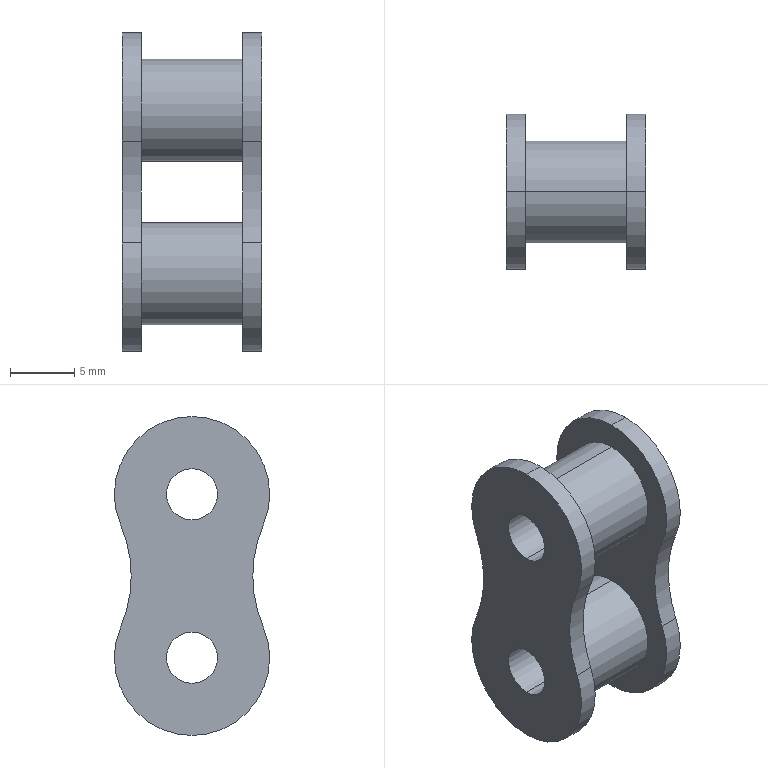Part | SolidWorks | features MoveFace 4, BaseBody 1, DelFace 1 | 1 solid | 22 faces | box 10.85 x 12.07 x 24.77 mm | volume 1258 mm3 | cylinder 18 | plane 4 | commonest cylinder face diameters 12.07 x6 3.98 x4 7.95 x4 20 x4
STEP:
#1=CARTESIAN_POINT('',(3.925,0.,3.975));
#2=VERTEX_POINT('',#1);
#3=CARTESIAN_POINT('',(3.925,0.,-3.975));
#4=VERTEX_POINT('',#3);
#5=CARTESIAN_POINT('',(3.925,0.,0.));
#6=DIRECTION('',(1.,0.,0.));
#7=DIRECTION('',(0.,0.,-1.));
#8=AXIS2_PLACEMENT_3D('',#5,#6,#7);
#9=CIRCLE('',#8,3.975);
#10=EDGE_CURVE('',#2,#4,#9,.T.);
#11=ORIENTED_EDGE('',*,*,#10,.F.);
#12=CARTESIAN_POINT('',(-3.925,0.,3.975));
#13=VERTEX_POINT('',#12);
#14=CARTESIAN_POINT('',(50.,0.,3.975));
#15=DIRECTION('',(-1.,0.,0.));
#16=VECTOR('',#15,1000.);
#17=LINE('',#14,#16);
#18=EDGE_CURVE('',#2,#13,#17,.T.);
#19=ORIENTED_EDGE('',*,*,#18,.T.);
#20=CARTESIAN_POINT('',(-3.925,0.,-3.975));
#21=VERTEX_POINT('',#20);
#22=CARTESIAN_POINT('',(-3.925,0.,0.));
#23=DIRECTION('',(1.,0.,0.));
#24=DIRECTION('',(0.,0.,-1.));
#25=AXIS2_PLACEMENT_3D('',#22,#23,#24);
#26=CIRCLE('',#25,3.975);
#27=EDGE_CURVE('',#13,#21,#26,.T.);
#28=ORIENTED_EDGE('',*,*,#27,.T.);
#29=CARTESIAN_POINT('',(50.,0.,-3.975));
#30=DIRECTION('',(-1.,0.,0.));
#31=VECTOR('',#30,1000.);
#32=LINE('',#29,#31);
#33=EDGE_CURVE('',#4,#21,#32,.T.);
#34=ORIENTED_EDGE('',*,*,#33,.F.);
#35=EDGE_LOOP('',(#11,#19,#28,#34));
#36=FACE_OUTER_BOUND('',#35,.T.);
#37=CARTESIAN_POINT('',(50.,0.,0.));
#38=DIRECTION('',(-1.,0.,0.));
#39=DIRECTION('',(0.,0.,-1.));
#40=AXIS2_PLACEMENT_3D('',#37,#38,#39);
#41=CYLINDRICAL_SURFACE('',#40,3.975);
#42=ADVANCED_FACE('',(#36),#41,.T.);
#43=CARTESIAN_POINT('',(3.925,0.,-8.725));
#44=VERTEX_POINT('',#43);
#45=CARTESIAN_POINT('',(3.925,0.,-16.675));
#46=VERTEX_POINT('',#45);
#47=CARTESIAN_POINT('',(3.925,0.,-12.7));
#48=DIRECTION('',(1.,0.,0.));
#49=DIRECTION('',(0.,0.,-1.));
#50=AXIS2_PLACEMENT_3D('',#47,#48,#49);
#51=CIRCLE('',#50,3.975);
#52=EDGE_CURVE('',#44,#46,#51,.T.);
#53=ORIENTED_EDGE('',*,*,#52,.F.);
#54=CARTESIAN_POINT('',(-3.925,0.,-8.725));
#55=VERTEX_POINT('',#54);
#56=CARTESIAN_POINT('',(50.,0.,-8.725));
#57=DIRECTION('',(-1.,0.,0.));
#58=VECTOR('',#57,1000.);
#59=LINE('',#56,#58);
#60=EDGE_CURVE('',#44,#55,#59,.T.);
#61=ORIENTED_EDGE('',*,*,#60,.T.);
#62=CARTESIAN_POINT('',(-3.925,0.,-16.675));
#63=VERTEX_POINT('',#62);
#64=CARTESIAN_POINT('',(-3.925,0.,-12.7));
#65=DIRECTION('',(1.,0.,0.));
#66=DIRECTION('',(0.,0.,-1.));
#67=AXIS2_PLACEMENT_3D('',#64,#65,#66);
#68=CIRCLE('',#67,3.975);
#69=EDGE_CURVE('',#55,#63,#68,.T.);
#70=ORIENTED_EDGE('',*,*,#69,.T.);
#71=CARTESIAN_POINT('',(50.,0.,-16.675));
#72=DIRECTION('',(-1.,0.,0.));
#73=VECTOR('',#72,1000.);
#74=LINE('',#71,#73);
#75=EDGE_CURVE('',#46,#63,#74,.T.);
#76=ORIENTED_EDGE('',*,*,#75,.F.);
#77=EDGE_LOOP('',(#53,#61,#70,#76));
#78=FACE_OUTER_BOUND('',#77,.T.);
#79=CARTESIAN_POINT('',(50.,0.,-12.7));
#80=DIRECTION('',(-1.,0.,0.));
#81=DIRECTION('',(0.,0.,-1.));
#82=AXIS2_PLACEMENT_3D('',#79,#80,#81);
#83=CYLINDRICAL_SURFACE('',#82,3.975);
#84=ADVANCED_FACE('',(#78),#83,.T.);
#85=CARTESIAN_POINT('',(-5.425,0.,-14.69));
#86=VERTEX_POINT('',#85);
#87=CARTESIAN_POINT('',(-5.425,0.,-10.71));
#88=VERTEX_POINT('',#87);
#89=CARTESIAN_POINT('',(-5.425,0.,-12.7));
#90=DIRECTION('',(1.,0.,0.));
#91=DIRECTION('',(0.,0.,-1.));
#92=AXIS2_PLACEMENT_3D('',#89,#90,#91);
#93=CIRCLE('',#92,1.99);
#94=EDGE_CURVE('',#86,#88,#93,.T.);
#95=ORIENTED_EDGE('',*,*,#94,.F.);
#96=CARTESIAN_POINT('',(5.425,0.,-14.69));
#97=VERTEX_POINT('',#96);
#98=CARTESIAN_POINT('',(5.925,0.,-14.69));
#99=DIRECTION('',(1.,0.,0.));
#100=VECTOR('',#99,1000.);
#101=LINE('',#98,#100);
#102=EDGE_CURVE('',#86,#97,#101,.T.);
#103=ORIENTED_EDGE('',*,*,#102,.T.);
#104=CARTESIAN_POINT('',(5.425,0.,-10.71));
#105=VERTEX_POINT('',#104);
#106=CARTESIAN_POINT('',(5.425,0.,-12.7));
#107=DIRECTION('',(1.,0.,0.));
#108=DIRECTION('',(0.,0.,-1.));
#109=AXIS2_PLACEMENT_3D('',#106,#107,#108);
#110=CIRCLE('',#109,1.99);
#111=EDGE_CURVE('',#97,#105,#110,.T.);
#112=ORIENTED_EDGE('',*,*,#111,.T.);
#113=CARTESIAN_POINT('',(5.925,0.,-10.71));
#114=DIRECTION('',(1.,0.,0.));
#115=VECTOR('',#114,1000.);
#116=LINE('',#113,#115);
#117=EDGE_CURVE('',#88,#105,#116,.T.);
#118=ORIENTED_EDGE('',*,*,#117,.F.);
#119=EDGE_LOOP('',(#95,#103,#112,#118));
#120=FACE_OUTER_BOUND('',#119,.T.);
#121=CARTESIAN_POINT('',(5.925,0.,-12.7));
#122=DIRECTION('',(1.,0.,0.));
#123=DIRECTION('',(0.,0.,1.));
#124=AXIS2_PLACEMENT_3D('',#121,#122,#123);
#125=CYLINDRICAL_SURFACE('',#124,1.99);
#126=ADVANCED_FACE('',(#120),#125,.F.);
#127=CARTESIAN_POINT('',(-5.425,0.,-1.99));
#128=VERTEX_POINT('',#127);
#129=CARTESIAN_POINT('',(-5.425,0.,1.99));
#130=VERTEX_POINT('',#129);
#131=CARTESIAN_POINT('',(-5.425,0.,0.));
#132=DIRECTION('',(1.,0.,0.));
#133=DIRECTION('',(0.,0.,-1.));
#134=AXIS2_PLACEMENT_3D('',#131,#132,#133);
#135=CIRCLE('',#134,1.99);
#136=EDGE_CURVE('',#128,#130,#135,.T.);
#137=ORIENTED_EDGE('',*,*,#136,.F.);
#138=CARTESIAN_POINT('',(5.425,0.,-1.99));
#139=VERTEX_POINT('',#138);
#140=CARTESIAN_POINT('',(5.925,0.,-1.99));
#141=DIRECTION('',(1.,0.,0.));
#142=VECTOR('',#141,1000.);
#143=LINE('',#140,#142);
#144=EDGE_CURVE('',#128,#139,#143,.T.);
#145=ORIENTED_EDGE('',*,*,#144,.T.);
#146=CARTESIAN_POINT('',(5.425,0.,1.99));
#147=VERTEX_POINT('',#146);
#148=CARTESIAN_POINT('',(5.425,0.,0.));
#149=DIRECTION('',(1.,0.,0.));
#150=DIRECTION('',(0.,0.,-1.));
#151=AXIS2_PLACEMENT_3D('',#148,#149,#150);
#152=CIRCLE('',#151,1.99);
#153=EDGE_CURVE('',#139,#147,#152,.T.);
#154=ORIENTED_EDGE('',*,*,#153,.T.);
#155=CARTESIAN_POINT('',(5.925,0.,1.99));
#156=DIRECTION('',(1.,0.,0.));
#157=VECTOR('',#156,1000.);
#158=LINE('',#155,#157);
#159=EDGE_CURVE('',#130,#147,#158,.T.);
#160=ORIENTED_EDGE('',*,*,#159,.F.);
#161=EDGE_LOOP('',(#137,#145,#154,#160));
#162=FACE_OUTER_BOUND('',#161,.T.);
#163=CARTESIAN_POINT('',(5.925,0.,0.));
#164=DIRECTION('',(1.,0.,0.));
#165=DIRECTION('',(0.,0.,1.));
#166=AXIS2_PLACEMENT_3D('',#163,#164,#165);
#167=CYLINDRICAL_SURFACE('',#166,1.99);
#168=ADVANCED_FACE('',(#162),#167,.F.);
#169=CARTESIAN_POINT('',(3.925,5.542,-2.39));
#170=VERTEX_POINT('',#169);
#171=CARTESIAN_POINT('',(3.925,0.,6.035));
#172=VERTEX_POINT('',#171);
#173=CARTESIAN_POINT('',(3.925,0.,0.));
#174=DIRECTION('',(1.,0.,0.));
#175=DIRECTION('',(0.,0.,-1.));
#176=AXIS2_PLACEMENT_3D('',#173,#174,#175);
#177=CIRCLE('',#176,6.035);
#178=EDGE_CURVE('',#170,#172,#177,.T.);
#179=ORIENTED_EDGE('',*,*,#178,.T.);
#180=CARTESIAN_POINT('',(5.425,0.,6.035));
#181=VERTEX_POINT('',#180);
#182=CARTESIAN_POINT('',(5.925,0.,6.035));
#183=DIRECTION('',(1.,0.,0.));
#184=VECTOR('',#183,1000.);
#185=LINE('',#182,#184);
#186=EDGE_CURVE('',#172,#181,#185,.T.);
#187=ORIENTED_EDGE('',*,*,#186,.T.);
#188=CARTESIAN_POINT('',(5.425,5.542,-2.39));
#189=VERTEX_POINT('',#188);
#190=CARTESIAN_POINT('',(5.425,0.,0.));
#191=DIRECTION('',(1.,0.,0.));
#192=DIRECTION('',(0.,0.,-1.));
#193=AXIS2_PLACEMENT_3D('',#190,#191,#192);
#194=CIRCLE('',#193,6.035);
#195=EDGE_CURVE('',#189,#181,#194,.T.);
#196=ORIENTED_EDGE('',*,*,#195,.F.);
#197=CARTESIAN_POINT('',(5.925,5.542,-2.39));
#198=DIRECTION('',(-1.,0.,0.));
#199=VECTOR('',#198,1000.);
#200=LINE('',#197,#199);
#201=EDGE_CURVE('',#189,#170,#200,.T.);
#202=ORIENTED_EDGE('',*,*,#201,.T.);
#203=EDGE_LOOP('',(#179,#187,#196,#202));
#204=FACE_OUTER_BOUND('',#203,.T.);
#205=CARTESIAN_POINT('',(5.925,0.,0.));
#206=DIRECTION('',(1.,0.,0.));
#207=DIRECTION('',(0.,0.,1.));
#208=AXIS2_PLACEMENT_3D('',#205,#206,#207);
#209=CYLINDRICAL_SURFACE('',#208,6.035);
#210=ADVANCED_FACE('',(#204),#209,.T.);
#211=CARTESIAN_POINT('',(-5.425,5.542,-2.39));
#212=VERTEX_POINT('',#211);
#213=CARTESIAN_POINT('',(-5.425,0.,6.035));
#214=VERTEX_POINT('',#213);
#215=CARTESIAN_POINT('',(-5.425,0.,0.));
#216=DIRECTION('',(1.,0.,0.));
#217=DIRECTION('',(0.,0.,-1.));
#218=AXIS2_PLACEMENT_3D('',#215,#216,#217);
#219=CIRCLE('',#218,6.035);
#220=EDGE_CURVE('',#212,#214,#219,.T.);
#221=ORIENTED_EDGE('',*,*,#220,.T.);
#222=CARTESIAN_POINT('',(-3.925,0.,6.035));
#223=VERTEX_POINT('',#222);
#224=CARTESIAN_POINT('',(5.925,0.,6.035));
#225=DIRECTION('',(1.,0.,0.));
#226=VECTOR('',#225,1000.);
#227=LINE('',#224,#226);
#228=EDGE_CURVE('',#214,#223,#227,.T.);
#229=ORIENTED_EDGE('',*,*,#228,.T.);
#230=CARTESIAN_POINT('',(-3.925,5.542,-2.39));
#231=VERTEX_POINT('',#230);
#232=CARTESIAN_POINT('',(-3.925,0.,0.));
#233=DIRECTION('',(1.,0.,0.));
#234=DIRECTION('',(0.,0.,-1.));
#235=AXIS2_PLACEMENT_3D('',#232,#233,#234);
#236=CIRCLE('',#235,6.035);
#237=EDGE_CURVE('',#231,#223,#236,.T.);
#238=ORIENTED_EDGE('',*,*,#237,.F.);
#239=CARTESIAN_POINT('',(5.925,5.542,-2.39));
#240=DIRECTION('',(-1.,0.,0.));
#241=VECTOR('',#240,1000.);
#242=LINE('',#239,#241);
#243=EDGE_CURVE('',#231,#212,#242,.T.);
#244=ORIENTED_EDGE('',*,*,#243,.T.);
#245=EDGE_LOOP('',(#221,#229,#238,#244));
#246=FACE_OUTER_BOUND('',#245,.T.);
#247=CARTESIAN_POINT('',(5.925,0.,0.));
#248=DIRECTION('',(1.,0.,0.));
#249=DIRECTION('',(0.,0.,1.));
#250=AXIS2_PLACEMENT_3D('',#247,#248,#249);
#251=CYLINDRICAL_SURFACE('',#250,6.035);
#252=ADVANCED_FACE('',(#246),#251,.T.);
#253=CARTESIAN_POINT('',(3.925,0.,0.));
#254=DIRECTION('',(1.,0.,0.));
#255=DIRECTION('',(0.,0.,-1.));
#256=AXIS2_PLACEMENT_3D('',#253,#254,#255);
#257=CIRCLE('',#256,3.975);
#258=EDGE_CURVE('',#4,#2,#257,.T.);
#259=ORIENTED_EDGE('',*,*,#258,.T.);
#260=ORIENTED_EDGE('',*,*,#10,.T.);
#261=EDGE_LOOP('',(#259,#260));
#262=FACE_BOUND('',#261,.T.);
#263=CARTESIAN_POINT('',(3.925,5.542,-10.31));
#264=VERTEX_POINT('',#263);
#265=CARTESIAN_POINT('',(3.925,14.724,-6.35));
#266=DIRECTION('',(1.,0.,0.));
#267=DIRECTION('',(0.,0.,-1.));
#268=AXIS2_PLACEMENT_3D('',#265,#266,#267);
#269=CIRCLE('',#268,10.);
#270=EDGE_CURVE('',#170,#264,#269,.T.);
#271=ORIENTED_EDGE('',*,*,#270,.T.);
#272=CARTESIAN_POINT('',(3.925,-5.542,-10.31));
#273=VERTEX_POINT('',#272);
#274=CARTESIAN_POINT('',(3.925,0.,-12.7));
#275=DIRECTION('',(1.,0.,0.));
#276=DIRECTION('',(0.,0.,-1.));
#277=AXIS2_PLACEMENT_3D('',#274,#275,#276);
#278=CIRCLE('',#277,6.035);
#279=EDGE_CURVE('',#273,#264,#278,.T.);
#280=ORIENTED_EDGE('',*,*,#279,.F.);
#281=CARTESIAN_POINT('',(3.925,-5.542,-2.39));
#282=VERTEX_POINT('',#281);
#283=CARTESIAN_POINT('',(3.925,-14.724,-6.35));
#284=DIRECTION('',(1.,0.,0.));
#285=DIRECTION('',(0.,0.,-1.));
#286=AXIS2_PLACEMENT_3D('',#283,#284,#285);
#287=CIRCLE('',#286,10.);
#288=EDGE_CURVE('',#273,#282,#287,.T.);
#289=ORIENTED_EDGE('',*,*,#288,.T.);
#290=CARTESIAN_POINT('',(3.925,0.,0.));
#291=DIRECTION('',(1.,0.,0.));
#292=DIRECTION('',(0.,0.,-1.));
#293=AXIS2_PLACEMENT_3D('',#290,#291,#292);
#294=CIRCLE('',#293,6.035);
#295=EDGE_CURVE('',#172,#282,#294,.T.);
#296=ORIENTED_EDGE('',*,*,#295,.F.);
#297=ORIENTED_EDGE('',*,*,#178,.F.);
#298=EDGE_LOOP('',(#271,#280,#289,#296,#297));
#299=FACE_OUTER_BOUND('',#298,.T.);
#300=CARTESIAN_POINT('',(3.925,0.,-12.7));
#301=DIRECTION('',(1.,0.,0.));
#302=DIRECTION('',(0.,0.,-1.));
#303=AXIS2_PLACEMENT_3D('',#300,#301,#302);
#304=CIRCLE('',#303,3.975);
#305=EDGE_CURVE('',#46,#44,#304,.T.);
#306=ORIENTED_EDGE('',*,*,#305,.T.);
#307=ORIENTED_EDGE('',*,*,#52,.T.);
#308=EDGE_LOOP('',(#306,#307));
#309=FACE_BOUND('',#308,.T.);
#310=CARTESIAN_POINT('',(3.925,7.362,-9.525));
#311=DIRECTION('',(1.,0.,0.));
#312=DIRECTION('',(0.,1.,0.));
#313=AXIS2_PLACEMENT_3D('',#310,#311,#312);
#314=PLANE('',#313);
#315=ADVANCED_FACE('',(#262,#299,#309),#314,.F.);
#316=ORIENTED_EDGE('',*,*,#228,.F.);
#317=CARTESIAN_POINT('',(-5.425,-5.542,-2.39));
#318=VERTEX_POINT('',#317);
#319=CARTESIAN_POINT('',(-5.425,0.,0.));
#320=DIRECTION('',(1.,0.,0.));
#321=DIRECTION('',(0.,0.,-1.));
#322=AXIS2_PLACEMENT_3D('',#319,#320,#321);
#323=CIRCLE('',#322,6.035);
#324=EDGE_CURVE('',#214,#318,#323,.T.);
#325=ORIENTED_EDGE('',*,*,#324,.T.);
#326=CARTESIAN_POINT('',(-3.925,-5.542,-2.39));
#327=VERTEX_POINT('',#326);
#328=CARTESIAN_POINT('',(5.925,-5.542,-2.39));
#329=DIRECTION('',(-1.,0.,0.));
#330=VECTOR('',#329,1000.);
#331=LINE('',#328,#330);
#332=EDGE_CURVE('',#327,#318,#331,.T.);
#333=ORIENTED_EDGE('',*,*,#332,.F.);
#334=CARTESIAN_POINT('',(-3.925,0.,0.));
#335=DIRECTION('',(1.,0.,0.));
#336=DIRECTION('',(0.,0.,-1.));
#337=AXIS2_PLACEMENT_3D('',#334,#335,#336);
#338=CIRCLE('',#337,6.035);
#339=EDGE_CURVE('',#223,#327,#338,.T.);
#340=ORIENTED_EDGE('',*,*,#339,.F.);
#341=EDGE_LOOP('',(#316,#325,#333,#340));
#342=FACE_OUTER_BOUND('',#341,.T.);
#343=CARTESIAN_POINT('',(5.925,0.,0.));
#344=DIRECTION('',(1.,0.,0.));
#345=DIRECTION('',(0.,0.,1.));
#346=AXIS2_PLACEMENT_3D('',#343,#344,#345);
#347=CYLINDRICAL_SURFACE('',#346,6.035);
#348=ADVANCED_FACE('',(#342),#347,.T.);
#349=ORIENTED_EDGE('',*,*,#270,.F.);
#350=ORIENTED_EDGE('',*,*,#201,.F.);
#351=CARTESIAN_POINT('',(5.425,5.542,-10.31));
#352=VERTEX_POINT('',#351);
#353=CARTESIAN_POINT('',(5.425,14.724,-6.35));
#354=DIRECTION('',(1.,0.,0.));
#355=DIRECTION('',(0.,0.,-1.));
#356=AXIS2_PLACEMENT_3D('',#353,#354,#355);
#357=CIRCLE('',#356,10.);
#358=EDGE_CURVE('',#189,#352,#357,.T.);
#359=ORIENTED_EDGE('',*,*,#358,.T.);
#360=CARTESIAN_POINT('',(5.925,5.542,-10.31));
#361=DIRECTION('',(-1.,0.,0.));
#362=VECTOR('',#361,1000.);
#363=LINE('',#360,#362);
#364=EDGE_CURVE('',#352,#264,#363,.T.);
#365=ORIENTED_EDGE('',*,*,#364,.T.);
#366=EDGE_LOOP('',(#349,#350,#359,#365));
#367=FACE_OUTER_BOUND('',#366,.T.);
#368=CARTESIAN_POINT('',(5.925,14.724,-6.35));
#369=DIRECTION('',(1.,0.,0.));
#370=DIRECTION('',(0.,0.,1.));
#371=AXIS2_PLACEMENT_3D('',#368,#369,#370);
#372=CYLINDRICAL_SURFACE('',#371,10.);
#373=ADVANCED_FACE('',(#367),#372,.F.);
#374=CARTESIAN_POINT('',(-3.925,-5.542,-10.31));
#375=VERTEX_POINT('',#374);
#376=CARTESIAN_POINT('',(-5.425,-5.542,-10.31));
#377=VERTEX_POINT('',#376);
#378=CARTESIAN_POINT('',(5.925,-5.542,-10.31));
#379=DIRECTION('',(-1.,0.,0.));
#380=VECTOR('',#379,1000.);
#381=LINE('',#378,#380);
#382=EDGE_CURVE('',#375,#377,#381,.T.);
#383=ORIENTED_EDGE('',*,*,#382,.F.);
#384=CARTESIAN_POINT('',(-3.925,-14.724,-6.35));
#385=DIRECTION('',(1.,0.,0.));
#386=DIRECTION('',(0.,0.,-1.));
#387=AXIS2_PLACEMENT_3D('',#384,#385,#386);
#388=CIRCLE('',#387,10.);
#389=EDGE_CURVE('',#375,#327,#388,.T.);
#390=ORIENTED_EDGE('',*,*,#389,.T.);
#391=ORIENTED_EDGE('',*,*,#332,.T.);
#392=CARTESIAN_POINT('',(-5.425,-14.724,-6.35));
#393=DIRECTION('',(1.,0.,0.));
#394=DIRECTION('',(0.,0.,-1.));
#395=AXIS2_PLACEMENT_3D('',#392,#393,#394);
#396=CIRCLE('',#395,10.);
#397=EDGE_CURVE('',#377,#318,#396,.T.);
#398=ORIENTED_EDGE('',*,*,#397,.F.);
#399=EDGE_LOOP('',(#383,#390,#391,#398));
#400=FACE_OUTER_BOUND('',#399,.T.);
#401=CARTESIAN_POINT('',(5.925,-14.724,-6.35));
#402=DIRECTION('',(1.,0.,0.));
#403=DIRECTION('',(0.,0.,1.));
#404=AXIS2_PLACEMENT_3D('',#401,#402,#403);
#405=CYLINDRICAL_SURFACE('',#404,10.);
#406=ADVANCED_FACE('',(#400),#405,.F.);
#407=ORIENTED_EDGE('',*,*,#186,.F.);
#408=ORIENTED_EDGE('',*,*,#295,.T.);
#409=CARTESIAN_POINT('',(5.425,-5.542,-2.39));
#410=VERTEX_POINT('',#409);
#411=CARTESIAN_POINT('',(5.925,-5.542,-2.39));
#412=DIRECTION('',(-1.,0.,0.));
#413=VECTOR('',#412,1000.);
#414=LINE('',#411,#413);
#415=EDGE_CURVE('',#410,#282,#414,.T.);
#416=ORIENTED_EDGE('',*,*,#415,.F.);
#417=CARTESIAN_POINT('',(5.425,0.,0.));
#418=DIRECTION('',(1.,0.,0.));
#419=DIRECTION('',(0.,0.,-1.));
#420=AXIS2_PLACEMENT_3D('',#417,#418,#419);
#421=CIRCLE('',#420,6.035);
#422=EDGE_CURVE('',#181,#410,#421,.T.);
#423=ORIENTED_EDGE('',*,*,#422,.F.);
#424=EDGE_LOOP('',(#407,#408,#416,#423));
#425=FACE_OUTER_BOUND('',#424,.T.);
#426=CARTESIAN_POINT('',(5.925,0.,0.));
#427=DIRECTION('',(1.,0.,0.));
#428=DIRECTION('',(0.,0.,1.));
#429=AXIS2_PLACEMENT_3D('',#426,#427,#428);
#430=CYLINDRICAL_SURFACE('',#429,6.035);
#431=ADVANCED_FACE('',(#425),#430,.T.);
#432=ORIENTED_EDGE('',*,*,#243,.F.);
#433=CARTESIAN_POINT('',(-3.925,5.542,-10.31));
#434=VERTEX_POINT('',#433);
#435=CARTESIAN_POINT('',(-3.925,14.724,-6.35));
#436=DIRECTION('',(1.,0.,0.));
#437=DIRECTION('',(0.,0.,-1.));
#438=AXIS2_PLACEMENT_3D('',#435,#436,#437);
#439=CIRCLE('',#438,10.);
#440=EDGE_CURVE('',#231,#434,#439,.T.);
#441=ORIENTED_EDGE('',*,*,#440,.T.);
#442=CARTESIAN_POINT('',(-5.425,5.542,-10.31));
#443=VERTEX_POINT('',#442);
#444=CARTESIAN_POINT('',(5.925,5.542,-10.31));
#445=DIRECTION('',(-1.,0.,0.));
#446=VECTOR('',#445,1000.);
#447=LINE('',#444,#446);
#448=EDGE_CURVE('',#434,#443,#447,.T.);
#449=ORIENTED_EDGE('',*,*,#448,.T.);
#450=CARTESIAN_POINT('',(-5.425,14.724,-6.35));
#451=DIRECTION('',(1.,0.,0.));
#452=DIRECTION('',(0.,0.,-1.));
#453=AXIS2_PLACEMENT_3D('',#450,#451,#452);
#454=CIRCLE('',#453,10.);
#455=EDGE_CURVE('',#212,#443,#454,.T.);
#456=ORIENTED_EDGE('',*,*,#455,.F.);
#457=EDGE_LOOP('',(#432,#441,#449,#456));
#458=FACE_OUTER_BOUND('',#457,.T.);
#459=CARTESIAN_POINT('',(5.925,14.724,-6.35));
#460=DIRECTION('',(1.,0.,0.));
#461=DIRECTION('',(0.,0.,1.));
#462=AXIS2_PLACEMENT_3D('',#459,#460,#461);
#463=CYLINDRICAL_SURFACE('',#462,10.);
#464=ADVANCED_FACE('',(#458),#463,.F.);
#465=CARTESIAN_POINT('',(-3.925,0.,-12.7));
#466=DIRECTION('',(1.,0.,0.));
#467=DIRECTION('',(0.,0.,-1.));
#468=AXIS2_PLACEMENT_3D('',#465,#466,#467);
#469=CIRCLE('',#468,6.035);
#470=EDGE_CURVE('',#375,#434,#469,.T.);
#471=ORIENTED_EDGE('',*,*,#470,.F.);
#472=ORIENTED_EDGE('',*,*,#382,.T.);
#473=CARTESIAN_POINT('',(-5.425,0.,-12.7));
#474=DIRECTION('',(1.,0.,0.));
#475=DIRECTION('',(0.,0.,-1.));
#476=AXIS2_PLACEMENT_3D('',#473,#474,#475);
#477=CIRCLE('',#476,6.035);
#478=EDGE_CURVE('',#377,#443,#477,.T.);
#479=ORIENTED_EDGE('',*,*,#478,.T.);
#480=ORIENTED_EDGE('',*,*,#448,.F.);
#481=EDGE_LOOP('',(#471,#472,#479,#480));
#482=FACE_OUTER_BOUND('',#481,.T.);
#483=CARTESIAN_POINT('',(5.925,0.,-12.7));
#484=DIRECTION('',(1.,0.,0.));
#485=DIRECTION('',(0.,0.,1.));
#486=AXIS2_PLACEMENT_3D('',#483,#484,#485);
#487=CYLINDRICAL_SURFACE('',#486,6.035);
#488=ADVANCED_FACE('',(#482),#487,.T.);
#489=CARTESIAN_POINT('',(5.425,-5.542,-10.31));
#490=VERTEX_POINT('',#489);
#491=CARTESIAN_POINT('',(5.925,-5.542,-10.31));
#492=DIRECTION('',(-1.,0.,0.));
#493=VECTOR('',#492,1000.);
#494=LINE('',#491,#493);
#495=EDGE_CURVE('',#490,#273,#494,.T.);
#496=ORIENTED_EDGE('',*,*,#495,.T.);
#497=ORIENTED_EDGE('',*,*,#279,.T.);
#498=ORIENTED_EDGE('',*,*,#364,.F.);
#499=CARTESIAN_POINT('',(5.425,0.,-12.7));
#500=DIRECTION('',(1.,0.,0.));
#501=DIRECTION('',(0.,0.,-1.));
#502=AXIS2_PLACEMENT_3D('',#499,#500,#501);
#503=CIRCLE('',#502,6.035);
#504=EDGE_CURVE('',#490,#352,#503,.T.);
#505=ORIENTED_EDGE('',*,*,#504,.F.);
#506=EDGE_LOOP('',(#496,#497,#498,#505));
#507=FACE_OUTER_BOUND('',#506,.T.);
#508=CARTESIAN_POINT('',(5.925,0.,-12.7));
#509=DIRECTION('',(1.,0.,0.));
#510=DIRECTION('',(0.,0.,1.));
#511=AXIS2_PLACEMENT_3D('',#508,#509,#510);
#512=CYLINDRICAL_SURFACE('',#511,6.035);
#513=ADVANCED_FACE('',(#507),#512,.T.);
#514=ORIENTED_EDGE('',*,*,#288,.F.);
#515=ORIENTED_EDGE('',*,*,#495,.F.);
#516=CARTESIAN_POINT('',(5.425,-14.724,-6.35));
#517=DIRECTION('',(1.,0.,0.));
#518=DIRECTION('',(0.,0.,-1.));
#519=AXIS2_PLACEMENT_3D('',#516,#517,#518);
#520=CIRCLE('',#519,10.);
#521=EDGE_CURVE('',#490,#410,#520,.T.);
#522=ORIENTED_EDGE('',*,*,#521,.T.);
#523=ORIENTED_EDGE('',*,*,#415,.T.);
#524=EDGE_LOOP('',(#514,#515,#522,#523));
#525=FACE_OUTER_BOUND('',#524,.T.);
#526=CARTESIAN_POINT('',(5.925,-14.724,-6.35));
#527=DIRECTION('',(1.,0.,0.));
#528=DIRECTION('',(0.,0.,1.));
#529=AXIS2_PLACEMENT_3D('',#526,#527,#528);
#530=CYLINDRICAL_SURFACE('',#529,10.);
#531=ADVANCED_FACE('',(#525),#530,.F.);
#532=CARTESIAN_POINT('',(-3.925,0.,0.));
#533=DIRECTION('',(1.,0.,0.));
#534=DIRECTION('',(0.,0.,-1.));
#535=AXIS2_PLACEMENT_3D('',#532,#533,#534);
#536=CIRCLE('',#535,3.975);
#537=EDGE_CURVE('',#21,#13,#536,.T.);
#538=ORIENTED_EDGE('',*,*,#537,.F.);
#539=ORIENTED_EDGE('',*,*,#27,.F.);
#540=EDGE_LOOP('',(#538,#539));
#541=FACE_BOUND('',#540,.T.);
#542=CARTESIAN_POINT('',(-3.925,0.,-12.7));
#543=DIRECTION('',(1.,0.,0.));
#544=DIRECTION('',(0.,0.,-1.));
#545=AXIS2_PLACEMENT_3D('',#542,#543,#544);
#546=CIRCLE('',#545,3.975);
#547=EDGE_CURVE('',#63,#55,#546,.T.);
#548=ORIENTED_EDGE('',*,*,#547,.F.);
#549=ORIENTED_EDGE('',*,*,#69,.F.);
#550=EDGE_LOOP('',(#548,#549));
#551=FACE_BOUND('',#550,.T.);
#552=ORIENTED_EDGE('',*,*,#440,.F.);
#553=ORIENTED_EDGE('',*,*,#237,.T.);
#554=ORIENTED_EDGE('',*,*,#339,.T.);
#555=ORIENTED_EDGE('',*,*,#389,.F.);
#556=ORIENTED_EDGE('',*,*,#470,.T.);
#557=EDGE_LOOP('',(#552,#553,#554,#555,#556));
#558=FACE_OUTER_BOUND('',#557,.T.);
#559=CARTESIAN_POINT('',(-3.925,7.362,-9.525));
#560=DIRECTION('',(1.,0.,0.));
#561=DIRECTION('',(0.,1.,0.));
#562=AXIS2_PLACEMENT_3D('',#559,#560,#561);
#563=PLANE('',#562);
#564=ADVANCED_FACE('',(#541,#551,#558),#563,.T.);
#565=ORIENTED_EDGE('',*,*,#358,.F.);
#566=ORIENTED_EDGE('',*,*,#195,.T.);
#567=ORIENTED_EDGE('',*,*,#422,.T.);
#568=ORIENTED_EDGE('',*,*,#521,.F.);
#569=ORIENTED_EDGE('',*,*,#504,.T.);
#570=EDGE_LOOP('',(#565,#566,#567,#568,#569));
#571=FACE_OUTER_BOUND('',#570,.T.);
#572=CARTESIAN_POINT('',(5.425,0.,-12.7));
#573=DIRECTION('',(1.,0.,0.));
#574=DIRECTION('',(0.,0.,-1.));
#575=AXIS2_PLACEMENT_3D('',#572,#573,#574);
#576=CIRCLE('',#575,1.99);
#577=EDGE_CURVE('',#105,#97,#576,.T.);
#578=ORIENTED_EDGE('',*,*,#577,.F.);
#579=ORIENTED_EDGE('',*,*,#111,.F.);
#580=EDGE_LOOP('',(#578,#579));
#581=FACE_BOUND('',#580,.T.);
#582=CARTESIAN_POINT('',(5.425,0.,0.));
#583=DIRECTION('',(1.,0.,0.));
#584=DIRECTION('',(0.,0.,-1.));
#585=AXIS2_PLACEMENT_3D('',#582,#583,#584);
#586=CIRCLE('',#585,1.99);
#587=EDGE_CURVE('',#147,#139,#586,.T.);
#588=ORIENTED_EDGE('',*,*,#587,.F.);
#589=ORIENTED_EDGE('',*,*,#153,.F.);
#590=EDGE_LOOP('',(#588,#589));
#591=FACE_BOUND('',#590,.T.);
#592=CARTESIAN_POINT('',(5.425,7.362,-9.525));
#593=DIRECTION('',(1.,0.,0.));
#594=DIRECTION('',(0.,1.,0.));
#595=AXIS2_PLACEMENT_3D('',#592,#593,#594);
#596=PLANE('',#595);
#597=ADVANCED_FACE('',(#571,#581,#591),#596,.T.);
#598=ORIENTED_EDGE('',*,*,#455,.T.);
#599=ORIENTED_EDGE('',*,*,#478,.F.);
#600=ORIENTED_EDGE('',*,*,#397,.T.);
#601=ORIENTED_EDGE('',*,*,#324,.F.);
#602=ORIENTED_EDGE('',*,*,#220,.F.);
#603=EDGE_LOOP('',(#598,#599,#600,#601,#602));
#604=FACE_OUTER_BOUND('',#603,.T.);
#605=CARTESIAN_POINT('',(-5.425,0.,-12.7));
#606=DIRECTION('',(1.,0.,0.));
#607=DIRECTION('',(0.,0.,-1.));
#608=AXIS2_PLACEMENT_3D('',#605,#606,#607);
#609=CIRCLE('',#608,1.99);
#610=EDGE_CURVE('',#88,#86,#609,.T.);
#611=ORIENTED_EDGE('',*,*,#610,.T.);
#612=ORIENTED_EDGE('',*,*,#94,.T.);
#613=EDGE_LOOP('',(#611,#612));
#614=FACE_BOUND('',#613,.T.);
#615=CARTESIAN_POINT('',(-5.425,0.,0.));
#616=DIRECTION('',(1.,0.,0.));
#617=DIRECTION('',(0.,0.,-1.));
#618=AXIS2_PLACEMENT_3D('',#615,#616,#617);
#619=CIRCLE('',#618,1.99);
#620=EDGE_CURVE('',#130,#128,#619,.T.);
#621=ORIENTED_EDGE('',*,*,#620,.T.);
#622=ORIENTED_EDGE('',*,*,#136,.T.);
#623=EDGE_LOOP('',(#621,#622));
#624=FACE_BOUND('',#623,.T.);
#625=CARTESIAN_POINT('',(-5.425,7.362,-9.525));
#626=DIRECTION('',(1.,0.,0.));
#627=DIRECTION('',(0.,1.,0.));
#628=AXIS2_PLACEMENT_3D('',#625,#626,#627);
#629=PLANE('',#628);
#630=ADVANCED_FACE('',(#604,#614,#624),#629,.F.);
#631=ORIENTED_EDGE('',*,*,#144,.F.);
#632=ORIENTED_EDGE('',*,*,#620,.F.);
#633=ORIENTED_EDGE('',*,*,#159,.T.);
#634=ORIENTED_EDGE('',*,*,#587,.T.);
#635=EDGE_LOOP('',(#631,#632,#633,#634));
#636=FACE_OUTER_BOUND('',#635,.T.);
#637=CARTESIAN_POINT('',(5.925,0.,0.));
#638=DIRECTION('',(1.,0.,0.));
#639=DIRECTION('',(0.,0.,1.));
#640=AXIS2_PLACEMENT_3D('',#637,#638,#639);
#641=CYLINDRICAL_SURFACE('',#640,1.99);
#642=ADVANCED_FACE('',(#636),#641,.F.);
#643=ORIENTED_EDGE('',*,*,#102,.F.);
#644=ORIENTED_EDGE('',*,*,#610,.F.);
#645=ORIENTED_EDGE('',*,*,#117,.T.);
#646=ORIENTED_EDGE('',*,*,#577,.T.);
#647=EDGE_LOOP('',(#643,#644,#645,#646));
#648=FACE_OUTER_BOUND('',#647,.T.);
#649=CARTESIAN_POINT('',(5.925,0.,-12.7));
#650=DIRECTION('',(1.,0.,0.));
#651=DIRECTION('',(0.,0.,1.));
#652=AXIS2_PLACEMENT_3D('',#649,#650,#651);
#653=CYLINDRICAL_SURFACE('',#652,1.99);
#654=ADVANCED_FACE('',(#648),#653,.F.);
#655=ORIENTED_EDGE('',*,*,#60,.F.);
#656=ORIENTED_EDGE('',*,*,#305,.F.);
#657=ORIENTED_EDGE('',*,*,#75,.T.);
#658=ORIENTED_EDGE('',*,*,#547,.T.);
#659=EDGE_LOOP('',(#655,#656,#657,#658));
#660=FACE_OUTER_BOUND('',#659,.T.);
#661=CARTESIAN_POINT('',(50.,0.,-12.7));
#662=DIRECTION('',(-1.,0.,0.));
#663=DIRECTION('',(0.,0.,-1.));
#664=AXIS2_PLACEMENT_3D('',#661,#662,#663);
#665=CYLINDRICAL_SURFACE('',#664,3.975);
#666=ADVANCED_FACE('',(#660),#665,.T.);
#667=ORIENTED_EDGE('',*,*,#18,.F.);
#668=ORIENTED_EDGE('',*,*,#258,.F.);
#669=ORIENTED_EDGE('',*,*,#33,.T.);
#670=ORIENTED_EDGE('',*,*,#537,.T.);
#671=EDGE_LOOP('',(#667,#668,#669,#670));
#672=FACE_OUTER_BOUND('',#671,.T.);
#673=CARTESIAN_POINT('',(50.,0.,0.));
#674=DIRECTION('',(-1.,0.,0.));
#675=DIRECTION('',(0.,0.,-1.));
#676=AXIS2_PLACEMENT_3D('',#673,#674,#675);
#677=CYLINDRICAL_SURFACE('',#676,3.975);
#678=ADVANCED_FACE('',(#672),#677,.T.);
#679=CLOSED_SHELL('',(#42,#84,#126,#168,#210,#252,#315,#348,#373,#406,#431,#464,#488,#513,#531,#564,#597,#630,#642,#654,#666,#678));
#680=MANIFOLD_SOLID_BREP('',#679);
#681=CARTESIAN_POINT('',(0.,0.,0.));
#682=DIRECTION('',(0.,0.,1.));
#683=DIRECTION('',(1.,0.,0.));
#684=AXIS2_PLACEMENT_3D('',#681,#682,#683);
#685=(LENGTH_UNIT()NAMED_UNIT(*)SI_UNIT(.MILLI.,.METRE.));
#686=UNCERTAINTY_MEASURE_WITH_UNIT(LENGTH_MEASURE(0.00001),#685,'','');
#687=(NAMED_UNIT(*)PLANE_ANGLE_UNIT()SI_UNIT($,.RADIAN.));
#688=(NAMED_UNIT(*)SI_UNIT($,.STERADIAN.)SOLID_ANGLE_UNIT());
#689=(GEOMETRIC_REPRESENTATION_CONTEXT(3)GLOBAL_UNCERTAINTY_ASSIGNED_CONTEXT((#686))GLOBAL_UNIT_ASSIGNED_CONTEXT((#685,#687,#688))REPRESENTATION_CONTEXT('',''));
#690=ADVANCED_BREP_SHAPE_REPRESENTATION('',(#680,#684),#689);